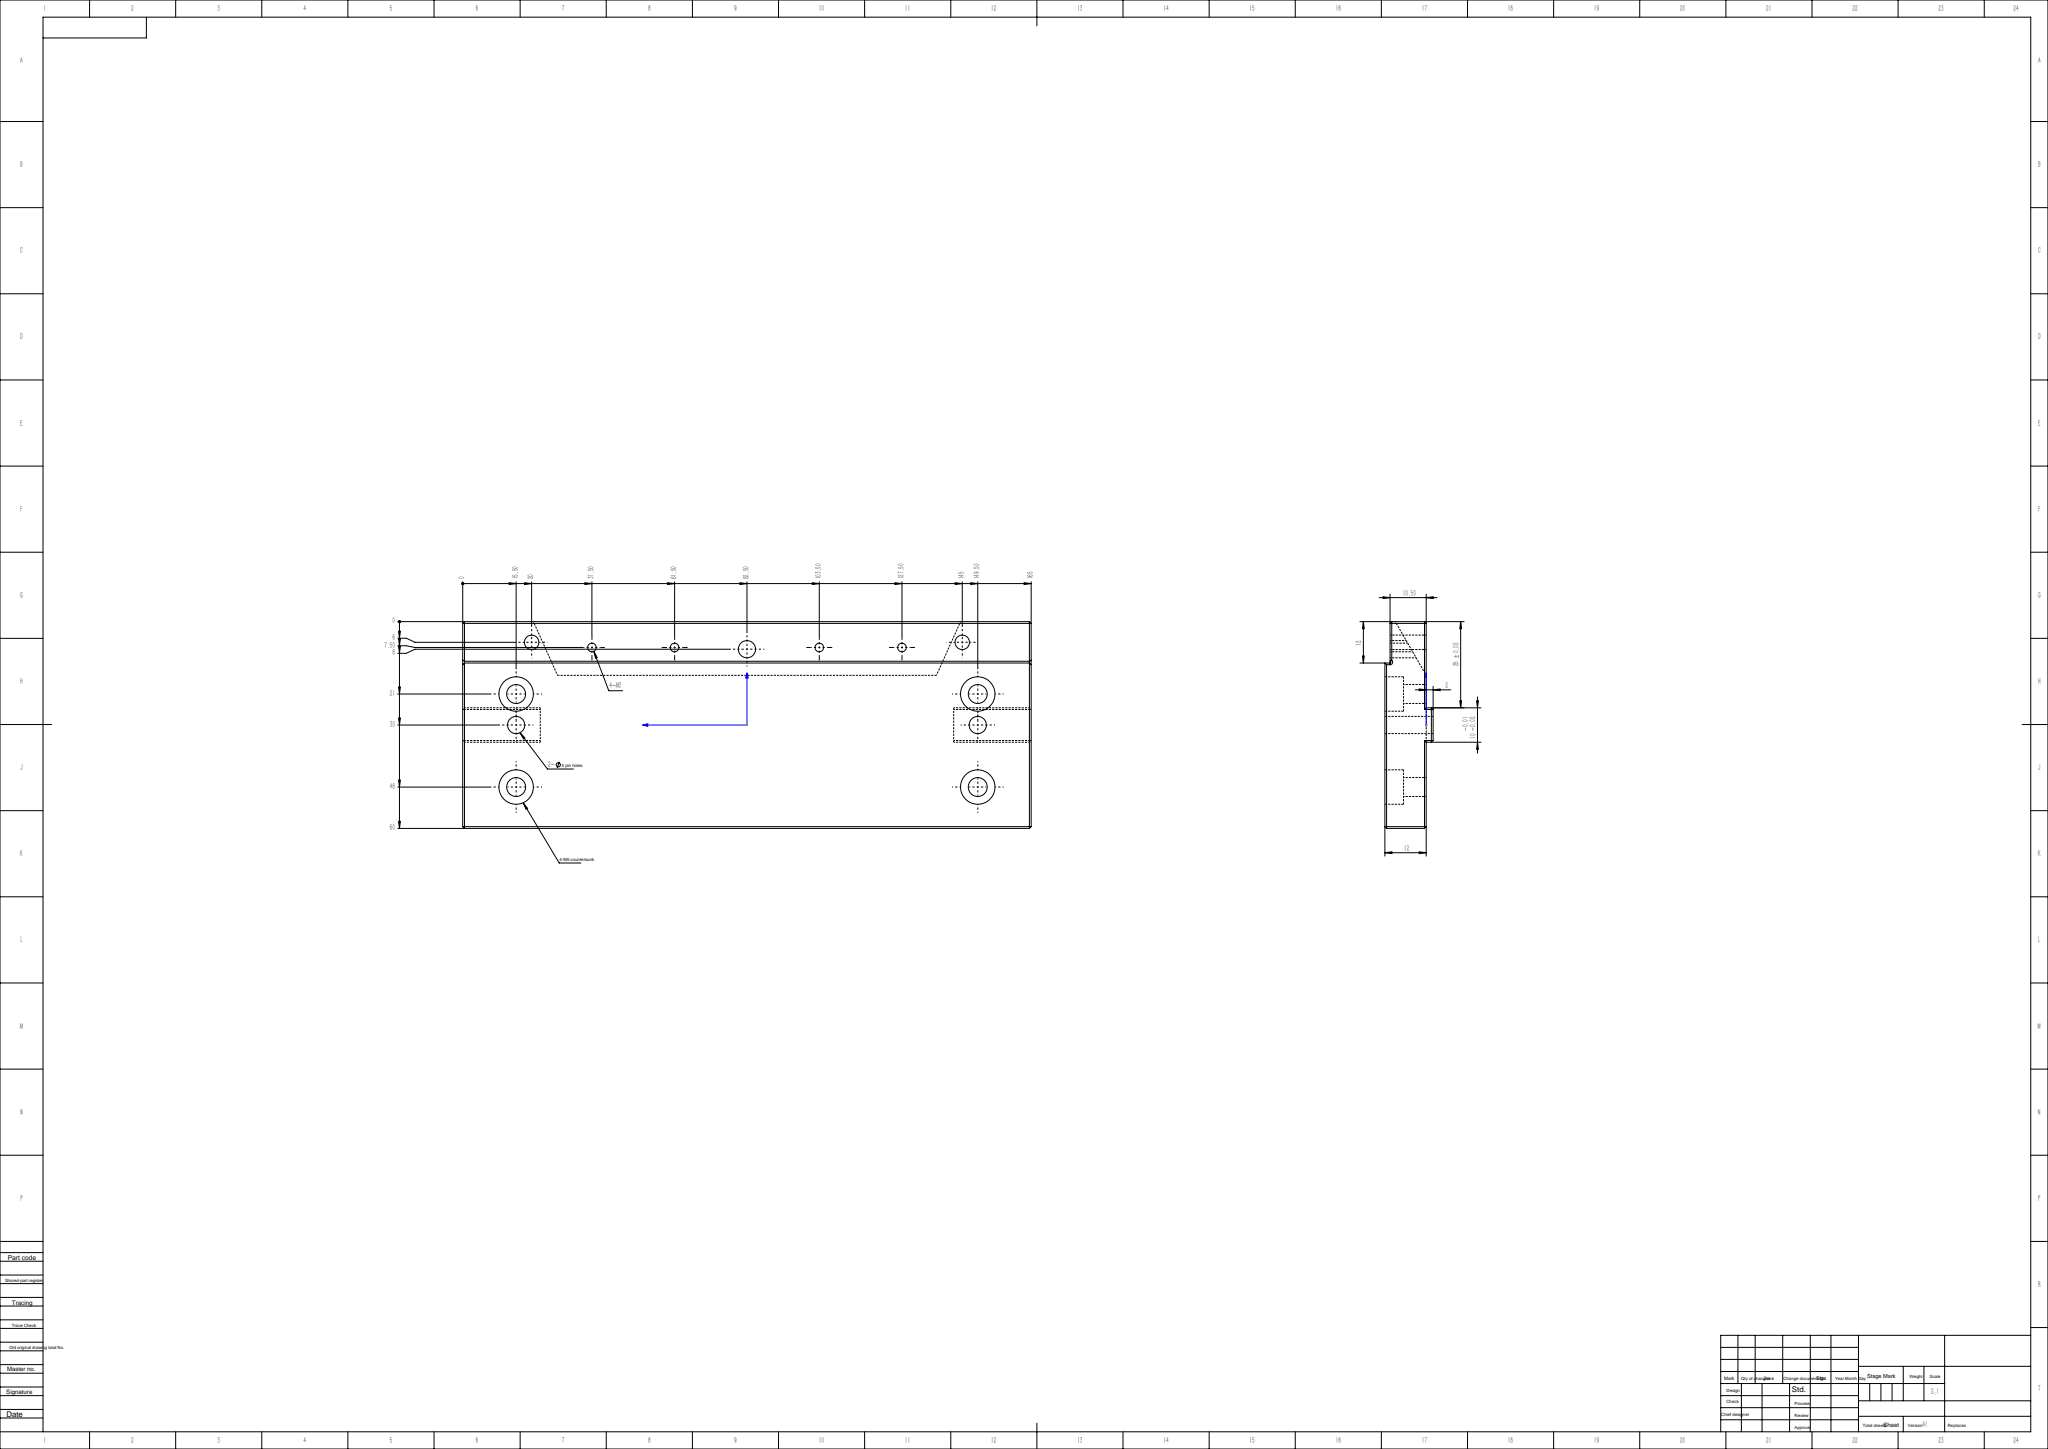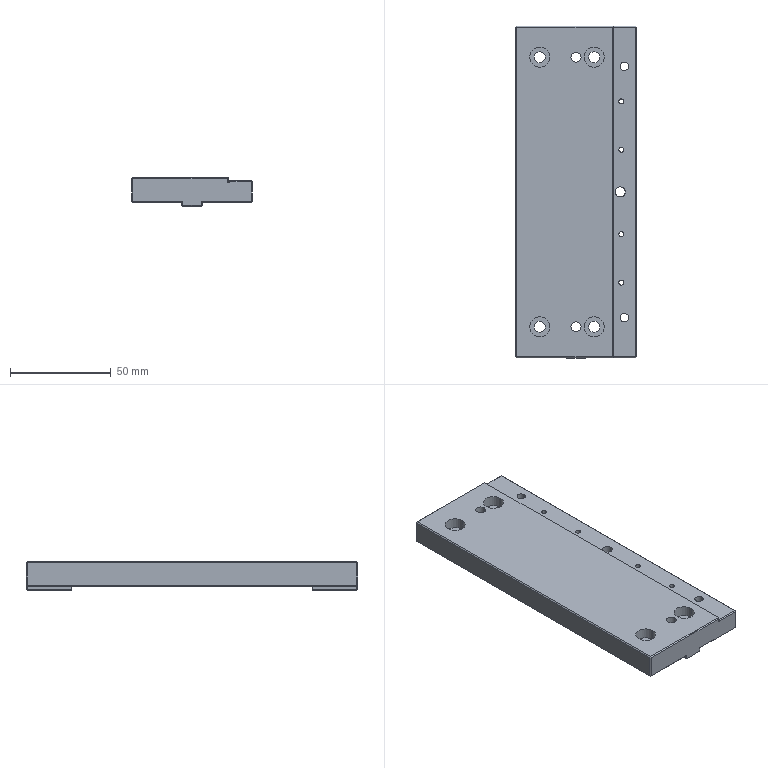Part | SolidWorks | features BaseBody 1 | 1 solid | 103 faces | box 60 x 165 x 14 mm | volume 104829 mm3 | plane 64 | cylinder 36 | cone 3 | commonest cylinder face diameters 2.5 x8 5.5 x8 10 x8 5 x6 4.2 x4 0.5 x2